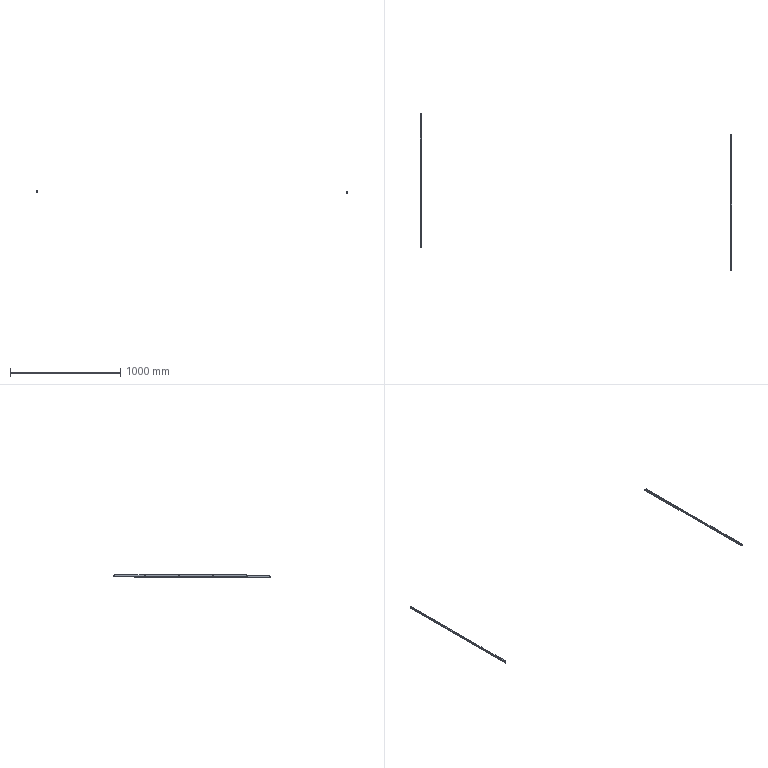NC program | NX | posted with a generic post | part box 2829 x 1430 x 20 mm
Whole program:
N10 G17 G21 G94 G90
(PLANAR_MILL , TOOL : D16-48-D16-100-3T-FINISH)
N12 T01 M6
N14 G53
N16 G17 G0 G90 X526.5 Y-0.499 B0. C0. S4000 M3
N18 G43 Z20. H1
N20 Z2.
N22 G94 G1 Z0. F1000.
N24 X513.5
N26 X-513.5
N28 X-526.5
N30 Z2.
N32 G0 Z20.
N34 M5
(动态粗 , TOOL : D8-25-D8-60-3T-ROUGH)
N36 T02 M6
N38 G53
N40 G17 G0 G90 X520.04 Y7.441 B0. C0. S6500 M3
N42 G43 Z20. H2
N44 Z-16.5
N46 G94 G1 X520.015 Y7.439 Z-16.656 F3000.
N48 X519.99 Y7.437 Z-16.718
N50 X519.965 Y7.435 Z-16.763
N52 X519.94 Y7.433 Z-16.8
N54 X519.915 Y7.431 Z-16.831
N56 X519.89 Y7.429 Z-16.857
N58 X519.865 Y7.427 Z-16.88
N60 X519.84 Y7.425 Z-16.9
N62 X519.815 Y7.423 Z-16.918
N64 X519.79 Y7.421 Z-16.933
N66 X519.765 Y7.419 Z-16.947
N68 X519.741 Y7.417 Z-16.958
N70 X519.716 Y7.415 Z-16.968
N72 X519.691 Y7.413 Z-16.977
N74 X519.666 Y7.411 Z-16.984
N76 X519.641 Y7.409 Z-16.99
N78 X519.616 Y7.407 Z-16.994
N80 X519.591 Y7.405 Z-16.997
N82 X519.566 Y7.403 Z-16.999
N84 X519.541 Y7.401 Z-17.
N86 X518.195 Y7.294
N88 G3 X517.545 Y6.866 R0.809
N90 X516.819 Y4.287 R7.111
N92 X516.521 Y-2.229 R60.108
N94 G1 X516.487 Y-5.285
N96 G2 X514.86 Y-8.098 R4.424
N98 X511.072 Y-9.843 R8.797
N100 X505.785 Y-10.403 R29.671
N102 X491.985 Y-10.497 R503.953
N104 G1 X-511.03 Y-10.496
N106 G2 X-514.017 Y-8.972 R4.211
N108 X-515.831 Y-5.15 R8.551
N110 X-516.397 Y0.062 R28.918
N112 X-516.464 Y5.31 R105.561
N114 X-514.683 Y8.246 R4.473
N116 X-510.933 Y9.877 R9.096
N118 X-505.792 Y10.405 R30.494
N120 X-491.992 Y10.5 R504.67
N122 G1 X511.072 Y10.498
N124 G2 X513.507 Y9.143 R3.606
N126 X514.752 Y6.875 R7.044
N128 X515.309 Y4.528 R6.87
N130 X515.476 Y-2.815 R63.569
N132 X515.2 Y-4.145 R11.568
N134 X515.095 Y-5.933 R8.778
N136 G1 X514.784 Y-6.821
N138 X514.284 Y-7.617
N140 X513.619 Y-8.282
N142 X512.822 Y-8.783
N144 X511.935 Y-9.093
N146 G2 X509.724 Y-9.199 R12.125
N148 X495.777 Y-9.492 R238.708
N150 G1 X489.627 Y-9.497
N152 X-508.329 Y-9.496
N154 G2 X-510.098 Y-9.206 R6.405
N156 X-511.935 Y-9.093 R9.752
N158 G1 X-512.822 Y-8.783
N160 X-513.619 Y-8.282
N162 X-514.284 Y-7.617
N164 X-514.784 Y-6.821
N166 X-515.095 Y-5.933
N168 G2 X-515.2 Y-3.723 R12.124
N170 X-515.418 Y2.693 R99.284
N172 X-515.2 Y3.961 R9.065
N174 X-515.095 Y5.936 R9.525
N176 G1 X-514.784 Y6.824
N178 X-514.284 Y7.62
N180 X-513.619 Y8.285
N182 X-512.822 Y8.785
N184 X-511.935 Y9.096
N186 G2 X-509.724 Y9.201 R12.125
N188 X-495.785 Y9.495 R238.621
N190 G1 X-489.635 Y9.499
N192 X508.021
N194 G2 X509.639 Y9.209 R5.811
N196 X511.935 Y9.096 R14.418
N198 G1 X512.822 Y8.785
N200 X513.619 Y8.285
N202 X514.284 Y7.62
N204 X514.784 Y6.824
N206 X515.095 Y5.936
N208 X515.2 Y5.001
N210 Y-5.
N212 X515.095 Y-5.933
N214 X514.784 Y-6.821
N216 X514.284 Y-7.617
N218 X513.619 Y-8.282
N220 X512.822 Y-8.783
N222 X511.935 Y-9.093
N224 G2 X509.724 Y-9.199 R12.125
N226 G1 X-511.001
N228 X-511.935 Y-9.093
N230 X-512.822 Y-8.783
N232 X-513.619 Y-8.282
N234 X-514.284 Y-7.617
N236 X-514.784 Y-6.821
N238 X-515.095 Y-5.933
N240 G2 X-515.2 Y-3.723 R12.124
N242 G1 Y5.002
N244 X-515.095 Y5.936
N246 X-514.784 Y6.824
N248 X-514.284 Y7.62
N250 X-513.619 Y8.285
N252 X-512.822 Y8.785
N254 X-511.935 Y9.096
N256 G2 X-509.724 Y9.201 R12.125
N258 G1 X509.751
N260 G3 X510.556 Y9.937 R0.808
N262 G1 X510.665 Y11.157
N264 X510.667 Y11.182 Z-16.999
N266 X510.669 Y11.207 Z-16.997
N268 X510.672 Y11.232 Z-16.994
N270 X510.674 Y11.257 Z-16.99
N272 X510.676 Y11.281 Z-16.984
N274 X510.678 Y11.306 Z-16.977
N276 X510.68 Y11.331 Z-16.968
N278 X510.683 Y11.356 Z-16.958
N280 X510.685 Y11.381 Z-16.947
N282 X510.687 Y11.406 Z-16.933
N284 X510.689 Y11.431 Z-16.918
N286 X510.692 Y11.456 Z-16.9
N288 X510.694 Y11.481 Z-16.88
N290 X510.696 Y11.506 Z-16.857
N292 X510.698 Y11.53 Z-16.831
N294 X510.701 Y11.555 Z-16.8
N296 X510.703 Y11.58 Z-16.763
N298 X510.705 Y11.605 Z-16.718
N300 X510.707 Y11.63 Z-16.656
N302 X510.709 Y11.655 Z-16.5
N304 G0 Z20.
N306 M5
(PLANAR_MILL_1 , TOOL : D8-25-D8-60-3T-FINISH)
N308 T03 M6
N310 G53
N312 G17 G0 G90 X-517.928 Y9.001 B0. C0. S4500 M3
N314 G43 Z20. H3
N316 Z-15.
N318 G94 G1 Z-17. F1000.
N320 X-510.996
N322 X515.
N324 Y-8.999
N326 X-515.
N328 Y4.997
N330 Y11.929
N332 Z-15.
N334 G0 Z20.
N336 M5
(PLANAR_MILL_1_COPY , TOOL : 倒角D6-90度)
N338 T04 M6
N340 G53
N342 G17 G0 G90 X-515.243 Y6.501 B0. C0. S4500 M3
N344 G43 Z20. H4
N346 Z0.5
N348 G94 G1 Z-1.5 F1000.
N350 X-510.997
N352 X512.5
N354 Y-6.499
N356 X-512.5
N358 Y4.999
N360 Y9.244
N362 Z0.5
N364 G0 Z20.
N366 M5
N368 M2